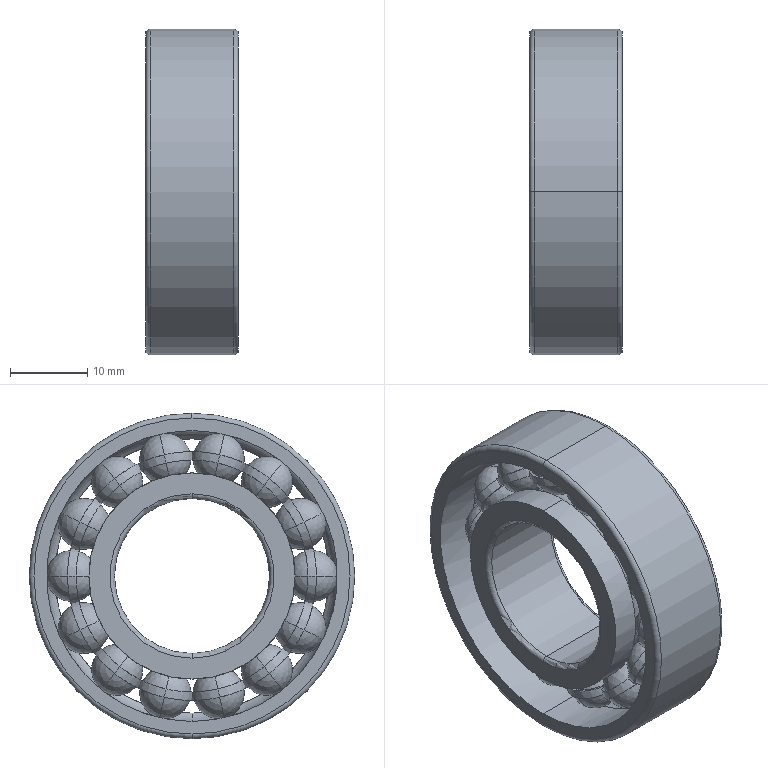Part | STEP file | angular contact ball bearing_68_iso_ISO 15 ABB - 1020 - Full,DE,AC,Full_68 | 1 solid | 254 faces | box 12 x 42 x 42 mm | volume 8271 mm3 | sphere 168 | torus 38 | plane 32 | cylinder 16 | commonest cylinder face diameters 20 x2 24.45 x2 26.6 x2 29.9 x2 32.1 x2 35.4 x2